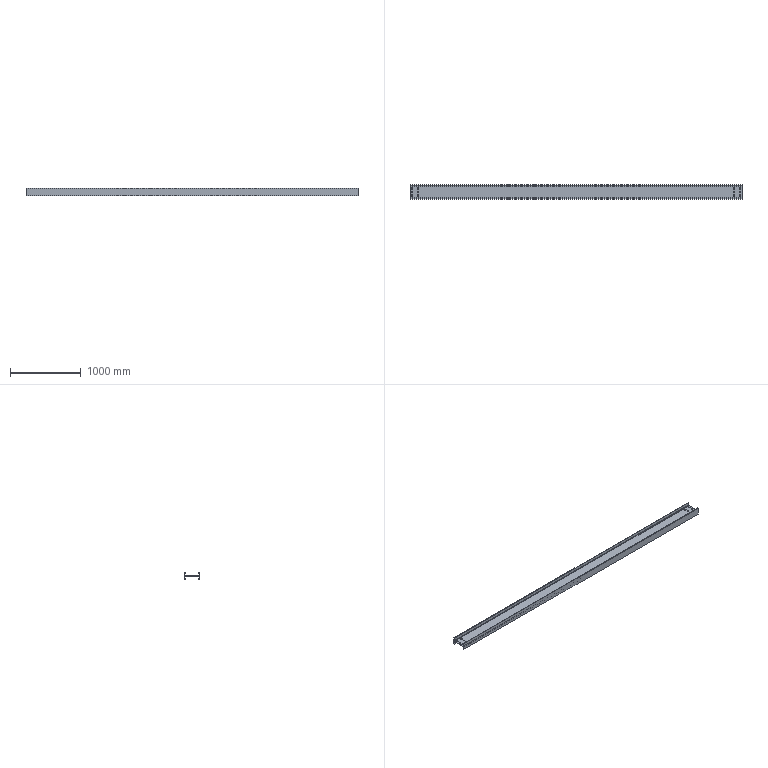Part | STEP file | 休息台主梁7主体_Default<As Machined> | 1 solid | 42 faces | box 4680 x 200 x 100 mm | volume 12462557 mm3 | cylinder 28 | plane 14 | commonest cylinder face diameters 19 x24 16 x4